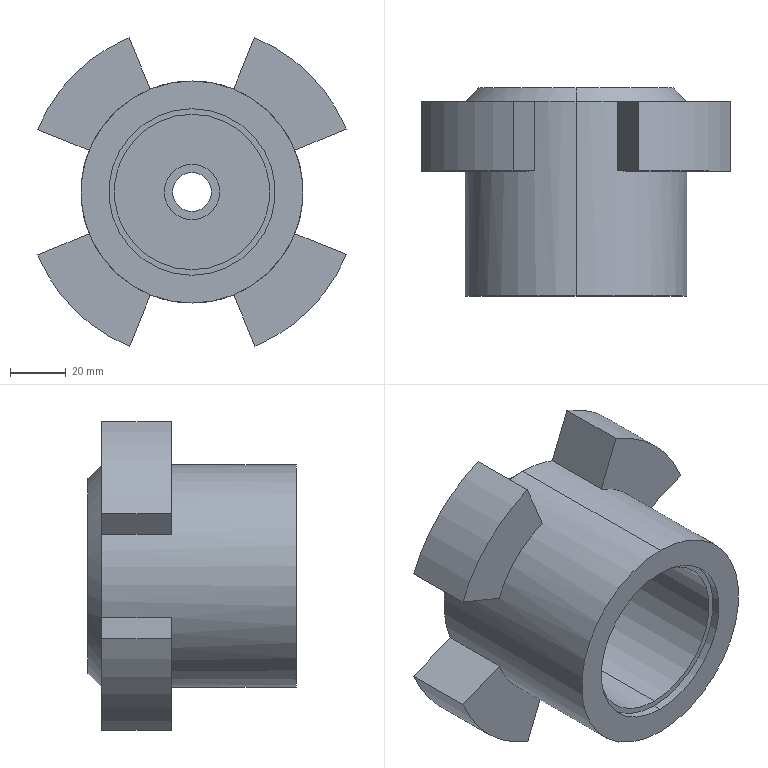Part | SolidWorks | features BaseBody 1 | 1 solid | 37 faces | box 111.243 x 75 x 111.243 mm | volume 319266 mm3 | plane 21 | cylinder 14 | cone 2 | commonest cylinder face diameters 120 x4 14 x2 20 x2 56 x2 60 x2 80 x2
STEP:
#1=CARTESIAN_POINT('',(0.,0.,40.));
#2=VERTEX_POINT('',#1);
#3=CARTESIAN_POINT('',(0.,0.,-40.));
#4=VERTEX_POINT('',#3);
#5=CARTESIAN_POINT('',(0.,0.,0.));
#6=DIRECTION('',(0.,1.,0.));
#7=DIRECTION('',(0.,0.,1.));
#8=AXIS2_PLACEMENT_3D('',#5,#6,#7);
#9=CIRCLE('',#8,40.);
#10=EDGE_CURVE('',#2,#4,#9,.T.);
#11=ORIENTED_EDGE('',*,*,#10,.T.);
#12=CARTESIAN_POINT('',(0.,70.,-40.));
#13=VERTEX_POINT('',#12);
#14=CARTESIAN_POINT('',(0.,45.,-40.));
#15=DIRECTION('',(0.,1.,0.));
#16=VECTOR('',#15,1000.);
#17=LINE('',#14,#16);
#18=EDGE_CURVE('',#4,#13,#17,.T.);
#19=ORIENTED_EDGE('',*,*,#18,.T.);
#20=CARTESIAN_POINT('',(15.,70.,-37.081));
#21=VERTEX_POINT('',#20);
#22=CARTESIAN_POINT('',(0.,70.,0.));
#23=DIRECTION('',(0.,-1.,0.));
#24=DIRECTION('',(0.,0.,1.));
#25=AXIS2_PLACEMENT_3D('',#22,#23,#24);
#26=CIRCLE('',#25,40.);
#27=EDGE_CURVE('',#13,#21,#26,.T.);
#28=ORIENTED_EDGE('',*,*,#27,.T.);
#29=CARTESIAN_POINT('',(15.,45.,-37.081));
#30=VERTEX_POINT('',#29);
#31=CARTESIAN_POINT('',(15.,45.,-37.081));
#32=DIRECTION('',(0.,-1.,0.));
#33=VECTOR('',#32,1000.);
#34=LINE('',#31,#33);
#35=EDGE_CURVE('',#21,#30,#34,.T.);
#36=ORIENTED_EDGE('',*,*,#35,.T.);
#37=CARTESIAN_POINT('',(37.081,45.,-15.));
#38=VERTEX_POINT('',#37);
#39=CARTESIAN_POINT('',(0.,45.,0.));
#40=DIRECTION('',(0.,-1.,0.));
#41=DIRECTION('',(0.,0.,1.));
#42=AXIS2_PLACEMENT_3D('',#39,#40,#41);
#43=CIRCLE('',#42,40.);
#44=EDGE_CURVE('',#30,#38,#43,.T.);
#45=ORIENTED_EDGE('',*,*,#44,.T.);
#46=CARTESIAN_POINT('',(37.081,70.,-15.));
#47=VERTEX_POINT('',#46);
#48=CARTESIAN_POINT('',(37.081,45.,-15.));
#49=DIRECTION('',(0.,1.,0.));
#50=VECTOR('',#49,1000.);
#51=LINE('',#48,#50);
#52=EDGE_CURVE('',#38,#47,#51,.T.);
#53=ORIENTED_EDGE('',*,*,#52,.T.);
#54=CARTESIAN_POINT('',(37.081,70.,15.));
#55=VERTEX_POINT('',#54);
#56=CARTESIAN_POINT('',(0.,70.,0.));
#57=DIRECTION('',(0.,-1.,0.));
#58=DIRECTION('',(0.,0.,1.));
#59=AXIS2_PLACEMENT_3D('',#56,#57,#58);
#60=CIRCLE('',#59,40.);
#61=EDGE_CURVE('',#47,#55,#60,.T.);
#62=ORIENTED_EDGE('',*,*,#61,.T.);
#63=CARTESIAN_POINT('',(37.081,45.,15.));
#64=VERTEX_POINT('',#63);
#65=CARTESIAN_POINT('',(37.081,45.,15.));
#66=DIRECTION('',(0.,-1.,0.));
#67=VECTOR('',#66,1000.);
#68=LINE('',#65,#67);
#69=EDGE_CURVE('',#55,#64,#68,.T.);
#70=ORIENTED_EDGE('',*,*,#69,.T.);
#71=CARTESIAN_POINT('',(15.,45.,37.081));
#72=VERTEX_POINT('',#71);
#73=CARTESIAN_POINT('',(0.,45.,0.));
#74=DIRECTION('',(0.,-1.,0.));
#75=DIRECTION('',(0.,0.,1.));
#76=AXIS2_PLACEMENT_3D('',#73,#74,#75);
#77=CIRCLE('',#76,40.);
#78=EDGE_CURVE('',#64,#72,#77,.T.);
#79=ORIENTED_EDGE('',*,*,#78,.T.);
#80=CARTESIAN_POINT('',(15.,70.,37.081));
#81=VERTEX_POINT('',#80);
#82=CARTESIAN_POINT('',(15.,45.,37.081));
#83=DIRECTION('',(0.,1.,0.));
#84=VECTOR('',#83,1000.);
#85=LINE('',#82,#84);
#86=EDGE_CURVE('',#72,#81,#85,.T.);
#87=ORIENTED_EDGE('',*,*,#86,.T.);
#88=CARTESIAN_POINT('',(0.,70.,40.));
#89=VERTEX_POINT('',#88);
#90=CARTESIAN_POINT('',(0.,70.,0.));
#91=DIRECTION('',(0.,-1.,0.));
#92=DIRECTION('',(0.,0.,1.));
#93=AXIS2_PLACEMENT_3D('',#90,#91,#92);
#94=CIRCLE('',#93,40.);
#95=EDGE_CURVE('',#81,#89,#94,.T.);
#96=ORIENTED_EDGE('',*,*,#95,.T.);
#97=CARTESIAN_POINT('',(0.,45.,40.));
#98=DIRECTION('',(0.,1.,0.));
#99=VECTOR('',#98,1000.);
#100=LINE('',#97,#99);
#101=EDGE_CURVE('',#2,#89,#100,.T.);
#102=ORIENTED_EDGE('',*,*,#101,.F.);
#103=EDGE_LOOP('',(#11,#19,#28,#36,#45,#53,#62,#70,#79,#87,#96,#102));
#104=FACE_OUTER_BOUND('',#103,.T.);
#105=CARTESIAN_POINT('',(0.,45.,0.));
#106=DIRECTION('',(0.,1.,0.));
#107=DIRECTION('',(0.,0.,1.));
#108=AXIS2_PLACEMENT_3D('',#105,#106,#107);
#109=CYLINDRICAL_SURFACE('',#108,40.);
#110=ADVANCED_FACE('',(#104),#109,.T.);
#111=CARTESIAN_POINT('',(0.,75.,-35.));
#112=VERTEX_POINT('',#111);
#113=CARTESIAN_POINT('',(0.,75.,35.));
#114=VERTEX_POINT('',#113);
#115=CARTESIAN_POINT('',(0.,75.,0.));
#116=DIRECTION('',(0.,-1.,0.));
#117=DIRECTION('',(0.,0.,-1.));
#118=AXIS2_PLACEMENT_3D('',#115,#116,#117);
#119=CIRCLE('',#118,35.);
#120=EDGE_CURVE('',#112,#114,#119,.T.);
#121=ORIENTED_EDGE('',*,*,#120,.T.);
#122=CARTESIAN_POINT('',(0.,70.,40.));
#123=DIRECTION('',(0.,-0.7071,0.7071));
#124=VECTOR('',#123,1000.);
#125=LINE('',#122,#124);
#126=EDGE_CURVE('',#114,#89,#125,.T.);
#127=ORIENTED_EDGE('',*,*,#126,.T.);
#128=ORIENTED_EDGE('',*,*,#95,.F.);
#129=CARTESIAN_POINT('',(0.,70.,0.));
#130=DIRECTION('',(0.,1.,0.));
#131=DIRECTION('',(0.,0.,-1.));
#132=AXIS2_PLACEMENT_3D('',#129,#130,#131);
#133=CIRCLE('',#132,40.);
#134=EDGE_CURVE('',#81,#55,#133,.T.);
#135=ORIENTED_EDGE('',*,*,#134,.T.);
#136=ORIENTED_EDGE('',*,*,#61,.F.);
#137=CARTESIAN_POINT('',(0.,70.,0.));
#138=DIRECTION('',(0.,1.,0.));
#139=DIRECTION('',(0.,0.,-1.));
#140=AXIS2_PLACEMENT_3D('',#137,#138,#139);
#141=CIRCLE('',#140,40.);
#142=EDGE_CURVE('',#47,#21,#141,.T.);
#143=ORIENTED_EDGE('',*,*,#142,.T.);
#144=ORIENTED_EDGE('',*,*,#27,.F.);
#145=CARTESIAN_POINT('',(0.,70.,-40.));
#146=DIRECTION('',(0.,-0.7071,-0.7071));
#147=VECTOR('',#146,1000.);
#148=LINE('',#145,#147);
#149=EDGE_CURVE('',#112,#13,#148,.T.);
#150=ORIENTED_EDGE('',*,*,#149,.F.);
#151=EDGE_LOOP('',(#121,#127,#128,#135,#136,#143,#144,#150));
#152=FACE_OUTER_BOUND('',#151,.T.);
#153=CARTESIAN_POINT('',(0.,70.,0.));
#154=DIRECTION('',(0.,-1.,0.));
#155=DIRECTION('',(0.,0.,-1.));
#156=AXIS2_PLACEMENT_3D('',#153,#154,#155);
#157=CONICAL_SURFACE('',#156,40.,0.7854);
#158=ADVANCED_FACE('',(#152),#157,.T.);
#159=CARTESIAN_POINT('',(0.,3.,30.));
#160=VERTEX_POINT('',#159);
#161=CARTESIAN_POINT('',(0.,3.,-30.));
#162=VERTEX_POINT('',#161);
#163=CARTESIAN_POINT('',(0.,3.,0.));
#164=DIRECTION('',(0.,-1.,0.));
#165=DIRECTION('',(0.,0.,-1.));
#166=AXIS2_PLACEMENT_3D('',#163,#164,#165);
#167=CIRCLE('',#166,30.);
#168=EDGE_CURVE('',#160,#162,#167,.T.);
#169=ORIENTED_EDGE('',*,*,#168,.F.);
#170=CARTESIAN_POINT('',(0.,0.,30.));
#171=VERTEX_POINT('',#170);
#172=CARTESIAN_POINT('',(0.,3.,30.));
#173=DIRECTION('',(0.,-1.,0.));
#174=VECTOR('',#173,1000.);
#175=LINE('',#172,#174);
#176=EDGE_CURVE('',#160,#171,#175,.T.);
#177=ORIENTED_EDGE('',*,*,#176,.T.);
#178=CARTESIAN_POINT('',(0.,0.,-30.));
#179=VERTEX_POINT('',#178);
#180=CARTESIAN_POINT('',(0.,0.,0.));
#181=DIRECTION('',(0.,-1.,0.));
#182=DIRECTION('',(0.,0.,-1.));
#183=AXIS2_PLACEMENT_3D('',#180,#181,#182);
#184=CIRCLE('',#183,30.);
#185=EDGE_CURVE('',#171,#179,#184,.T.);
#186=ORIENTED_EDGE('',*,*,#185,.T.);
#187=CARTESIAN_POINT('',(0.,3.,-30.));
#188=DIRECTION('',(0.,-1.,0.));
#189=VECTOR('',#188,1000.);
#190=LINE('',#187,#189);
#191=EDGE_CURVE('',#162,#179,#190,.T.);
#192=ORIENTED_EDGE('',*,*,#191,.F.);
#193=EDGE_LOOP('',(#169,#177,#186,#192));
#194=FACE_OUTER_BOUND('',#193,.T.);
#195=CARTESIAN_POINT('',(0.,3.,0.));
#196=DIRECTION('',(0.,-1.,0.));
#197=DIRECTION('',(0.,0.,-1.));
#198=AXIS2_PLACEMENT_3D('',#195,#196,#197);
#199=CYLINDRICAL_SURFACE('',#198,30.);
#200=ADVANCED_FACE('',(#194),#199,.F.);
#201=CARTESIAN_POINT('',(0.,51.,-7.));
#202=VERTEX_POINT('',#201);
#203=CARTESIAN_POINT('',(0.,51.,7.));
#204=VERTEX_POINT('',#203);
#205=CARTESIAN_POINT('',(0.,51.,0.));
#206=DIRECTION('',(0.,1.,0.));
#207=DIRECTION('',(0.,0.,1.));
#208=AXIS2_PLACEMENT_3D('',#205,#206,#207);
#209=CIRCLE('',#208,7.);
#210=EDGE_CURVE('',#202,#204,#209,.T.);
#211=ORIENTED_EDGE('',*,*,#210,.F.);
#212=CARTESIAN_POINT('',(0.,75.,-7.));
#213=VERTEX_POINT('',#212);
#214=CARTESIAN_POINT('',(0.,75.,-7.));
#215=DIRECTION('',(0.,1.,0.));
#216=VECTOR('',#215,1000.);
#217=LINE('',#214,#216);
#218=EDGE_CURVE('',#202,#213,#217,.T.);
#219=ORIENTED_EDGE('',*,*,#218,.T.);
#220=CARTESIAN_POINT('',(0.,75.,7.));
#221=VERTEX_POINT('',#220);
#222=CARTESIAN_POINT('',(0.,75.,0.));
#223=DIRECTION('',(0.,-1.,0.));
#224=DIRECTION('',(0.,0.,1.));
#225=AXIS2_PLACEMENT_3D('',#222,#223,#224);
#226=CIRCLE('',#225,7.);
#227=EDGE_CURVE('',#221,#213,#226,.T.);
#228=ORIENTED_EDGE('',*,*,#227,.F.);
#229=CARTESIAN_POINT('',(0.,75.,7.));
#230=DIRECTION('',(0.,1.,0.));
#231=VECTOR('',#230,1000.);
#232=LINE('',#229,#231);
#233=EDGE_CURVE('',#204,#221,#232,.T.);
#234=ORIENTED_EDGE('',*,*,#233,.F.);
#235=EDGE_LOOP('',(#211,#219,#228,#234));
#236=FACE_OUTER_BOUND('',#235,.T.);
#237=CARTESIAN_POINT('',(0.,75.,0.));
#238=DIRECTION('',(0.,1.,0.));
#239=DIRECTION('',(0.,0.,1.));
#240=AXIS2_PLACEMENT_3D('',#237,#238,#239);
#241=CYLINDRICAL_SURFACE('',#240,7.);
#242=ADVANCED_FACE('',(#236),#241,.F.);
#243=CARTESIAN_POINT('',(0.,53.,28.));
#244=VERTEX_POINT('',#243);
#245=CARTESIAN_POINT('',(0.,53.,-28.));
#246=VERTEX_POINT('',#245);
#247=CARTESIAN_POINT('',(0.,53.,0.));
#248=DIRECTION('',(0.,-1.,0.));
#249=DIRECTION('',(0.,0.,-1.));
#250=AXIS2_PLACEMENT_3D('',#247,#248,#249);
#251=CIRCLE('',#250,28.);
#252=EDGE_CURVE('',#244,#246,#251,.T.);
#253=ORIENTED_EDGE('',*,*,#252,.F.);
#254=CARTESIAN_POINT('',(0.,3.,28.));
#255=VERTEX_POINT('',#254);
#256=CARTESIAN_POINT('',(0.,51.,28.));
#257=DIRECTION('',(0.,-1.,0.));
#258=VECTOR('',#257,1000.);
#259=LINE('',#256,#258);
#260=EDGE_CURVE('',#244,#255,#259,.T.);
#261=ORIENTED_EDGE('',*,*,#260,.T.);
#262=CARTESIAN_POINT('',(0.,3.,-28.));
#263=VERTEX_POINT('',#262);
#264=CARTESIAN_POINT('',(0.,3.,0.));
#265=DIRECTION('',(0.,1.,0.));
#266=DIRECTION('',(0.,0.,-1.));
#267=AXIS2_PLACEMENT_3D('',#264,#265,#266);
#268=CIRCLE('',#267,28.);
#269=EDGE_CURVE('',#263,#255,#268,.T.);
#270=ORIENTED_EDGE('',*,*,#269,.F.);
#271=CARTESIAN_POINT('',(0.,51.,-28.));
#272=DIRECTION('',(0.,-1.,0.));
#273=VECTOR('',#272,1000.);
#274=LINE('',#271,#273);
#275=EDGE_CURVE('',#246,#263,#274,.T.);
#276=ORIENTED_EDGE('',*,*,#275,.F.);
#277=EDGE_LOOP('',(#253,#261,#270,#276));
#278=FACE_OUTER_BOUND('',#277,.T.);
#279=CARTESIAN_POINT('',(0.,51.,0.));
#280=DIRECTION('',(0.,-1.,0.));
#281=DIRECTION('',(0.,0.,-1.));
#282=AXIS2_PLACEMENT_3D('',#279,#280,#281);
#283=CYLINDRICAL_SURFACE('',#282,28.);
#284=ADVANCED_FACE('',(#278),#283,.F.);
#285=CARTESIAN_POINT('',(0.,53.,-10.));
#286=VERTEX_POINT('',#285);
#287=CARTESIAN_POINT('',(0.,53.,10.));
#288=VERTEX_POINT('',#287);
#289=CARTESIAN_POINT('',(0.,53.,0.));
#290=DIRECTION('',(0.,-1.,0.));
#291=DIRECTION('',(0.,0.,-1.));
#292=AXIS2_PLACEMENT_3D('',#289,#290,#291);
#293=CIRCLE('',#292,10.);
#294=EDGE_CURVE('',#286,#288,#293,.T.);
#295=ORIENTED_EDGE('',*,*,#294,.T.);
#296=CARTESIAN_POINT('',(0.,51.,10.));
#297=VERTEX_POINT('',#296);
#298=CARTESIAN_POINT('',(0.,53.,10.));
#299=DIRECTION('',(0.,-1.,0.));
#300=VECTOR('',#299,1000.);
#301=LINE('',#298,#300);
#302=EDGE_CURVE('',#288,#297,#301,.T.);
#303=ORIENTED_EDGE('',*,*,#302,.T.);
#304=CARTESIAN_POINT('',(0.,51.,-10.));
#305=VERTEX_POINT('',#304);
#306=CARTESIAN_POINT('',(0.,51.,0.));
#307=DIRECTION('',(0.,-1.,0.));
#308=DIRECTION('',(0.,0.,-1.));
#309=AXIS2_PLACEMENT_3D('',#306,#307,#308);
#310=CIRCLE('',#309,10.);
#311=EDGE_CURVE('',#305,#297,#310,.T.);
#312=ORIENTED_EDGE('',*,*,#311,.F.);
#313=CARTESIAN_POINT('',(0.,53.,-10.));
#314=DIRECTION('',(0.,-1.,0.));
#315=VECTOR('',#314,1000.);
#316=LINE('',#313,#315);
#317=EDGE_CURVE('',#286,#305,#316,.T.);
#318=ORIENTED_EDGE('',*,*,#317,.F.);
#319=EDGE_LOOP('',(#295,#303,#312,#318));
#320=FACE_OUTER_BOUND('',#319,.T.);
#321=CARTESIAN_POINT('',(0.,53.,0.));
#322=DIRECTION('',(0.,-1.,0.));
#323=DIRECTION('',(0.,0.,-1.));
#324=AXIS2_PLACEMENT_3D('',#321,#322,#323);
#325=CYLINDRICAL_SURFACE('',#324,10.);
#326=ADVANCED_FACE('',(#320),#325,.T.);
#327=ORIENTED_EDGE('',*,*,#18,.F.);
#328=CARTESIAN_POINT('',(0.,0.,0.));
#329=DIRECTION('',(0.,1.,0.));
#330=DIRECTION('',(0.,0.,1.));
#331=AXIS2_PLACEMENT_3D('',#328,#329,#330);
#332=CIRCLE('',#331,40.);
#333=EDGE_CURVE('',#4,#2,#332,.T.);
#334=ORIENTED_EDGE('',*,*,#333,.T.);
#335=ORIENTED_EDGE('',*,*,#101,.T.);
#336=CARTESIAN_POINT('',(-15.,70.,37.081));
#337=VERTEX_POINT('',#336);
#338=CARTESIAN_POINT('',(0.,70.,0.));
#339=DIRECTION('',(0.,-1.,0.));
#340=DIRECTION('',(0.,0.,1.));
#341=AXIS2_PLACEMENT_3D('',#338,#339,#340);
#342=CIRCLE('',#341,40.);
#343=EDGE_CURVE('',#89,#337,#342,.T.);
#344=ORIENTED_EDGE('',*,*,#343,.T.);
#345=CARTESIAN_POINT('',(-15.,45.,37.081));
#346=VERTEX_POINT('',#345);
#347=CARTESIAN_POINT('',(-15.,45.,37.081));
#348=DIRECTION('',(0.,-1.,0.));
#349=VECTOR('',#348,1000.);
#350=LINE('',#347,#349);
#351=EDGE_CURVE('',#337,#346,#350,.T.);
#352=ORIENTED_EDGE('',*,*,#351,.T.);
#353=CARTESIAN_POINT('',(-37.081,45.,15.));
#354=VERTEX_POINT('',#353);
#355=CARTESIAN_POINT('',(0.,45.,0.));
#356=DIRECTION('',(0.,-1.,0.));
#357=DIRECTION('',(0.,0.,1.));
#358=AXIS2_PLACEMENT_3D('',#355,#356,#357);
#359=CIRCLE('',#358,40.);
#360=EDGE_CURVE('',#346,#354,#359,.T.);
#361=ORIENTED_EDGE('',*,*,#360,.T.);
#362=CARTESIAN_POINT('',(-37.081,70.,15.));
#363=VERTEX_POINT('',#362);
#364=CARTESIAN_POINT('',(-37.081,45.,15.));
#365=DIRECTION('',(0.,1.,0.));
#366=VECTOR('',#365,1000.);
#367=LINE('',#364,#366);
#368=EDGE_CURVE('',#354,#363,#367,.T.);
#369=ORIENTED_EDGE('',*,*,#368,.T.);
#370=CARTESIAN_POINT('',(-37.081,70.,-15.));
#371=VERTEX_POINT('',#370);
#372=CARTESIAN_POINT('',(0.,70.,0.));
#373=DIRECTION('',(0.,-1.,0.));
#374=DIRECTION('',(0.,0.,1.));
#375=AXIS2_PLACEMENT_3D('',#372,#373,#374);
#376=CIRCLE('',#375,40.);
#377=EDGE_CURVE('',#363,#371,#376,.T.);
#378=ORIENTED_EDGE('',*,*,#377,.T.);
#379=CARTESIAN_POINT('',(-37.081,45.,-15.));
#380=VERTEX_POINT('',#379);
#381=CARTESIAN_POINT('',(-37.081,45.,-15.));
#382=DIRECTION('',(0.,-1.,0.));
#383=VECTOR('',#382,1000.);
#384=LINE('',#381,#383);
#385=EDGE_CURVE('',#371,#380,#384,.T.);
#386=ORIENTED_EDGE('',*,*,#385,.T.);
#387=CARTESIAN_POINT('',(-15.,45.,-37.081));
#388=VERTEX_POINT('',#387);
#389=CARTESIAN_POINT('',(0.,45.,0.));
#390=DIRECTION('',(0.,-1.,0.));
#391=DIRECTION('',(0.,0.,1.));
#392=AXIS2_PLACEMENT_3D('',#389,#390,#391);
#393=CIRCLE('',#392,40.);
#394=EDGE_CURVE('',#380,#388,#393,.T.);
#395=ORIENTED_EDGE('',*,*,#394,.T.);
#396=CARTESIAN_POINT('',(-15.,70.,-37.081));
#397=VERTEX_POINT('',#396);
#398=CARTESIAN_POINT('',(-15.,45.,-37.081));
#399=DIRECTION('',(0.,1.,0.));
#400=VECTOR('',#399,1000.);
#401=LINE('',#398,#400);
#402=EDGE_CURVE('',#388,#397,#401,.T.);
#403=ORIENTED_EDGE('',*,*,#402,.T.);
#404=CARTESIAN_POINT('',(0.,70.,0.));
#405=DIRECTION('',(0.,-1.,0.));
#406=DIRECTION('',(0.,0.,1.));
#407=AXIS2_PLACEMENT_3D('',#404,#405,#406);
#408=CIRCLE('',#407,40.);
#409=EDGE_CURVE('',#397,#13,#408,.T.);
#410=ORIENTED_EDGE('',*,*,#409,.T.);
#411=EDGE_LOOP('',(#327,#334,#335,#344,#352,#361,#369,#378,#386,#395,#403,#410));
#412=FACE_OUTER_BOUND('',#411,.T.);
#413=CARTESIAN_POINT('',(0.,45.,0.));
#414=DIRECTION('',(0.,1.,0.));
#415=DIRECTION('',(0.,0.,1.));
#416=AXIS2_PLACEMENT_3D('',#413,#414,#415);
#417=CYLINDRICAL_SURFACE('',#416,40.);
#418=ADVANCED_FACE('',(#412),#417,.T.);
#419=ORIENTED_EDGE('',*,*,#126,.F.);
#420=CARTESIAN_POINT('',(0.,75.,0.));
#421=DIRECTION('',(0.,-1.,0.));
#422=DIRECTION('',(0.,0.,-1.));
#423=AXIS2_PLACEMENT_3D('',#420,#421,#422);
#424=CIRCLE('',#423,35.);
#425=EDGE_CURVE('',#114,#112,#424,.T.);
#426=ORIENTED_EDGE('',*,*,#425,.T.);
#427=ORIENTED_EDGE('',*,*,#149,.T.);
#428=ORIENTED_EDGE('',*,*,#409,.F.);
#429=CARTESIAN_POINT('',(0.,70.,0.));
#430=DIRECTION('',(0.,1.,0.));
#431=DIRECTION('',(0.,0.,-1.));
#432=AXIS2_PLACEMENT_3D('',#429,#430,#431);
#433=CIRCLE('',#432,40.);
#434=EDGE_CURVE('',#397,#371,#433,.T.);
#435=ORIENTED_EDGE('',*,*,#434,.T.);
#436=ORIENTED_EDGE('',*,*,#377,.F.);
#437=CARTESIAN_POINT('',(0.,70.,0.));
#438=DIRECTION('',(0.,1.,0.));
#439=DIRECTION('',(0.,0.,-1.));
#440=AXIS2_PLACEMENT_3D('',#437,#438,#439);
#441=CIRCLE('',#440,40.);
#442=EDGE_CURVE('',#363,#337,#441,.T.);
#443=ORIENTED_EDGE('',*,*,#442,.T.);
#444=ORIENTED_EDGE('',*,*,#343,.F.);
#445=EDGE_LOOP('',(#419,#426,#427,#428,#435,#436,#443,#444));
#446=FACE_OUTER_BOUND('',#445,.T.);
#447=CARTESIAN_POINT('',(0.,70.,0.));
#448=DIRECTION('',(0.,-1.,0.));
#449=DIRECTION('',(0.,0.,-1.));
#450=AXIS2_PLACEMENT_3D('',#447,#448,#449);
#451=CONICAL_SURFACE('',#450,40.,0.7854);
#452=ADVANCED_FACE('',(#446),#451,.T.);
#453=ORIENTED_EDGE('',*,*,#402,.F.);
#454=CARTESIAN_POINT('',(-22.5,45.,-55.621));
#455=VERTEX_POINT('',#454);
#456=CARTESIAN_POINT('',(-22.5,45.,-55.621));
#457=DIRECTION('',(0.375,0.,0.927));
#458=VECTOR('',#457,1000.);
#459=LINE('',#456,#458);
#460=EDGE_CURVE('',#455,#388,#459,.T.);
#461=ORIENTED_EDGE('',*,*,#460,.F.);
#462=CARTESIAN_POINT('',(-22.5,70.,-55.621));
#463=VERTEX_POINT('',#462);
#464=CARTESIAN_POINT('',(-22.5,45.,-55.621));
#465=DIRECTION('',(0.,-1.,0.));
#466=VECTOR('',#465,1000.);
#467=LINE('',#464,#466);
#468=EDGE_CURVE('',#463,#455,#467,.T.);
#469=ORIENTED_EDGE('',*,*,#468,.F.);
#470=CARTESIAN_POINT('',(-22.5,70.,-55.621));
#471=DIRECTION('',(-0.375,0.,-0.927));
#472=VECTOR('',#471,1000.);
#473=LINE('',#470,#472);
#474=EDGE_CURVE('',#397,#463,#473,.T.);
#475=ORIENTED_EDGE('',*,*,#474,.F.);
#476=EDGE_LOOP('',(#453,#461,#469,#475));
#477=FACE_OUTER_BOUND('',#476,.T.);
#478=CARTESIAN_POINT('',(-22.5,45.,-55.621));
#479=DIRECTION('',(-0.927,0.,0.375));
#480=DIRECTION('',(0.375,0.,0.927));
#481=AXIS2_PLACEMENT_3D('',#478,#479,#480);
#482=PLANE('',#481);
#483=ADVANCED_FACE('',(#477),#482,.F.);
#484=ORIENTED_EDGE('',*,*,#394,.F.);
#485=CARTESIAN_POINT('',(-55.54,45.,-22.7));
#486=VERTEX_POINT('',#485);
#487=CARTESIAN_POINT('',(-37.081,45.,-15.));
#488=DIRECTION('',(-0.9229,0.,-0.385));
#489=VECTOR('',#488,1000.);
#490=LINE('',#487,#489);
#491=EDGE_CURVE('',#380,#486,#490,.T.);
#492=ORIENTED_EDGE('',*,*,#491,.T.);
#493=CARTESIAN_POINT('',(0.,45.,0.));
#494=DIRECTION('',(0.,-1.,0.));
#495=DIRECTION('',(0.,0.,-1.));
#496=AXIS2_PLACEMENT_3D('',#493,#494,#495);
#497=CIRCLE('',#496,60.);
#498=EDGE_CURVE('',#486,#455,#497,.T.);
#499=ORIENTED_EDGE('',*,*,#498,.T.);
#500=ORIENTED_EDGE('',*,*,#460,.T.);
#501=EDGE_LOOP('',(#484,#492,#499,#500));
#502=FACE_OUTER_BOUND('',#501,.T.);
#503=CARTESIAN_POINT('',(0.,45.,0.));
#504=DIRECTION('',(0.,-1.,0.));
#505=DIRECTION('',(0.,0.,-1.));
#506=AXIS2_PLACEMENT_3D('',#503,#504,#505);
#507=PLANE('',#506);
#508=ADVANCED_FACE('',(#502),#507,.T.);
#509=CARTESIAN_POINT('',(-55.54,70.,-22.7));
#510=VERTEX_POINT('',#509);
#511=CARTESIAN_POINT('',(-55.54,45.,-22.7));
#512=DIRECTION('',(0.,1.,0.));
#513=VECTOR('',#512,1000.);
#514=LINE('',#511,#513);
#515=EDGE_CURVE('',#486,#510,#514,.T.);
#516=ORIENTED_EDGE('',*,*,#515,.F.);
#517=ORIENTED_EDGE('',*,*,#491,.F.);
#518=ORIENTED_EDGE('',*,*,#385,.F.);
#519=CARTESIAN_POINT('',(-55.54,70.,-22.7));
#520=DIRECTION('',(0.9229,0.,0.385));
#521=VECTOR('',#520,1000.);
#522=LINE('',#519,#521);
#523=EDGE_CURVE('',#510,#371,#522,.T.);
#524=ORIENTED_EDGE('',*,*,#523,.F.);
#525=EDGE_LOOP('',(#516,#517,#518,#524));
#526=FACE_OUTER_BOUND('',#525,.T.);
#527=CARTESIAN_POINT('',(-55.54,45.,-22.7));
#528=DIRECTION('',(0.385,0.,-0.9229));
#529=DIRECTION('',(-0.9229,0.,-0.385));
#530=AXIS2_PLACEMENT_3D('',#527,#528,#529);
#531=PLANE('',#530);
#532=ADVANCED_FACE('',(#526),#531,.F.);
#533=ORIENTED_EDGE('',*,*,#368,.F.);
#534=CARTESIAN_POINT('',(-55.621,45.,22.5));
#535=VERTEX_POINT('',#534);
#536=CARTESIAN_POINT('',(-55.621,45.,22.5));
#537=DIRECTION('',(0.927,0.,-0.375));
#538=VECTOR('',#537,1000.);
#539=LINE('',#536,#538);
#540=EDGE_CURVE('',#535,#354,#539,.T.);
#541=ORIENTED_EDGE('',*,*,#540,.F.);
#542=CARTESIAN_POINT('',(-55.621,70.,22.5));
#543=VERTEX_POINT('',#542);
#544=CARTESIAN_POINT('',(-55.621,45.,22.5));
#545=DIRECTION('',(0.,-1.,0.));
#546=VECTOR('',#545,1000.);
#547=LINE('',#544,#546);
#548=EDGE_CURVE('',#543,#535,#547,.T.);
#549=ORIENTED_EDGE('',*,*,#548,.F.);
#550=CARTESIAN_POINT('',(-55.621,70.,22.5));
#551=DIRECTION('',(-0.927,0.,0.375));
#552=VECTOR('',#551,1000.);
#553=LINE('',#550,#552);
#554=EDGE_CURVE('',#363,#543,#553,.T.);
#555=ORIENTED_EDGE('',*,*,#554,.F.);
#556=EDGE_LOOP('',(#533,#541,#549,#555));
#557=FACE_OUTER_BOUND('',#556,.T.);
#558=CARTESIAN_POINT('',(-55.621,45.,22.5));
#559=DIRECTION('',(0.375,0.,0.927));
#560=DIRECTION('',(0.927,0.,-0.375));
#561=AXIS2_PLACEMENT_3D('',#558,#559,#560);
#562=PLANE('',#561);
#563=ADVANCED_FACE('',(#557),#562,.F.);
#564=ORIENTED_EDGE('',*,*,#360,.F.);
#565=CARTESIAN_POINT('',(-22.7,45.,55.54));
#566=VERTEX_POINT('',#565);
#567=CARTESIAN_POINT('',(-15.,45.,37.081));
#568=DIRECTION('',(-0.385,0.,0.9229));
#569=VECTOR('',#568,1000.);
#570=LINE('',#567,#569);
#571=EDGE_CURVE('',#346,#566,#570,.T.);
#572=ORIENTED_EDGE('',*,*,#571,.T.);
#573=CARTESIAN_POINT('',(0.,45.,0.));
#574=DIRECTION('',(0.,-1.,0.));
#575=DIRECTION('',(0.,0.,-1.));
#576=AXIS2_PLACEMENT_3D('',#573,#574,#575);
#577=CIRCLE('',#576,60.);
#578=EDGE_CURVE('',#566,#535,#577,.T.);
#579=ORIENTED_EDGE('',*,*,#578,.T.);
#580=ORIENTED_EDGE('',*,*,#540,.T.);
#581=EDGE_LOOP('',(#564,#572,#579,#580));
#582=FACE_OUTER_BOUND('',#581,.T.);
#583=CARTESIAN_POINT('',(0.,45.,0.));
#584=DIRECTION('',(0.,-1.,0.));
#585=DIRECTION('',(0.,0.,-1.));
#586=AXIS2_PLACEMENT_3D('',#583,#584,#585);
#587=PLANE('',#586);
#588=ADVANCED_FACE('',(#582),#587,.T.);
#589=CARTESIAN_POINT('',(-22.7,70.,55.54));
#590=VERTEX_POINT('',#589);
#591=CARTESIAN_POINT('',(-22.7,45.,55.54));
#592=DIRECTION('',(0.,1.,0.));
#593=VECTOR('',#592,1000.);
#594=LINE('',#591,#593);
#595=EDGE_CURVE('',#566,#590,#594,.T.);
#596=ORIENTED_EDGE('',*,*,#595,.F.);
#597=ORIENTED_EDGE('',*,*,#571,.F.);
#598=ORIENTED_EDGE('',*,*,#351,.F.);
#599=CARTESIAN_POINT('',(-22.7,70.,55.54));
#600=DIRECTION('',(0.385,0.,-0.9229));
#601=VECTOR('',#600,1000.);
#602=LINE('',#599,#601);
#603=EDGE_CURVE('',#590,#337,#602,.T.);
#604=ORIENTED_EDGE('',*,*,#603,.F.);
#605=EDGE_LOOP('',(#596,#597,#598,#604));
#606=FACE_OUTER_BOUND('',#605,.T.);
#607=CARTESIAN_POINT('',(-22.7,45.,55.54));
#608=DIRECTION('',(-0.9229,0.,-0.385));
#609=DIRECTION('',(-0.385,0.,0.9229));
#610=AXIS2_PLACEMENT_3D('',#607,#608,#609);
#611=PLANE('',#610);
#612=ADVANCED_FACE('',(#606),#611,.F.);
#613=CARTESIAN_POINT('',(0.,0.,0.));
#614=DIRECTION('',(0.,-1.,0.));
#615=DIRECTION('',(0.,0.,-1.));
#616=AXIS2_PLACEMENT_3D('',#613,#614,#615);
#617=CIRCLE('',#616,30.);
#618=EDGE_CURVE('',#179,#171,#617,.T.);
#619=ORIENTED_EDGE('',*,*,#618,.F.);
#620=ORIENTED_EDGE('',*,*,#185,.F.);
#621=EDGE_LOOP('',(#619,#620));
#622=FACE_BOUND('',#621,.T.);
#623=ORIENTED_EDGE('',*,*,#10,.F.);
#624=ORIENTED_EDGE('',*,*,#333,.F.);
#625=EDGE_LOOP('',(#623,#624));
#626=FACE_OUTER_BOUND('',#625,.T.);
#627=CARTESIAN_POINT('',(0.,0.,0.));
#628=DIRECTION('',(0.,1.,0.));
#629=DIRECTION('',(0.,0.,1.));
#630=AXIS2_PLACEMENT_3D('',#627,#628,#629);
#631=PLANE('',#630);
#632=ADVANCED_FACE('',(#622,#626),#631,.F.);
#633=ORIENTED_EDGE('',*,*,#603,.T.);
#634=ORIENTED_EDGE('',*,*,#442,.F.);
#635=ORIENTED_EDGE('',*,*,#554,.T.);
#636=CARTESIAN_POINT('',(0.,70.,0.));
#637=DIRECTION('',(0.,1.,0.));
#638=DIRECTION('',(0.,0.,-1.));
#639=AXIS2_PLACEMENT_3D('',#636,#637,#638);
#640=CIRCLE('',#639,60.);
#641=EDGE_CURVE('',#543,#590,#640,.T.);
#642=ORIENTED_EDGE('',*,*,#641,.T.);
#643=EDGE_LOOP('',(#633,#634,#635,#642));
#644=FACE_OUTER_BOUND('',#643,.T.);
#645=CARTESIAN_POINT('',(0.,70.,0.));
#646=DIRECTION('',(0.,1.,0.));
#647=DIRECTION('',(0.,0.,1.));
#648=AXIS2_PLACEMENT_3D('',#645,#646,#647);
#649=PLANE('',#648);
#650=ADVANCED_FACE('',(#644),#649,.T.);
#651=ORIENTED_EDGE('',*,*,#523,.T.);
#652=ORIENTED_EDGE('',*,*,#434,.F.);
#653=ORIENTED_EDGE('',*,*,#474,.T.);
#654=CARTESIAN_POINT('',(0.,70.,0.));
#655=DIRECTION('',(0.,1.,0.));
#656=DIRECTION('',(0.,0.,-1.));
#657=AXIS2_PLACEMENT_3D('',#654,#655,#656);
#658=CIRCLE('',#657,60.);
#659=EDGE_CURVE('',#463,#510,#658,.T.);
#660=ORIENTED_EDGE('',*,*,#659,.T.);
#661=EDGE_LOOP('',(#651,#652,#653,#660));
#662=FACE_OUTER_BOUND('',#661,.T.);
#663=CARTESIAN_POINT('',(0.,70.,0.));
#664=DIRECTION('',(0.,1.,0.));
#665=DIRECTION('',(0.,0.,1.));
#666=AXIS2_PLACEMENT_3D('',#663,#664,#665);
#667=PLANE('',#666);
#668=ADVANCED_FACE('',(#662),#667,.T.);
#669=ORIENTED_EDGE('',*,*,#227,.T.);
#670=CARTESIAN_POINT('',(0.,75.,0.));
#671=DIRECTION('',(0.,-1.,0.));
#672=DIRECTION('',(0.,0.,1.));
#673=AXIS2_PLACEMENT_3D('',#670,#671,#672);
#674=CIRCLE('',#673,7.);
#675=EDGE_CURVE('',#213,#221,#674,.T.);
#676=ORIENTED_EDGE('',*,*,#675,.T.);
#677=EDGE_LOOP('',(#669,#676));
#678=FACE_BOUND('',#677,.T.);
#679=ORIENTED_EDGE('',*,*,#120,.F.);
#680=ORIENTED_EDGE('',*,*,#425,.F.);
#681=EDGE_LOOP('',(#679,#680));
#682=FACE_OUTER_BOUND('',#681,.T.);
#683=CARTESIAN_POINT('',(0.,75.,0.));
#684=DIRECTION('',(0.,1.,0.));
#685=DIRECTION('',(0.,0.,1.));
#686=AXIS2_PLACEMENT_3D('',#683,#684,#685);
#687=PLANE('',#686);
#688=ADVANCED_FACE('',(#678,#682),#687,.T.);
#689=ORIENTED_EDGE('',*,*,#659,.F.);
#690=ORIENTED_EDGE('',*,*,#468,.T.);
#691=ORIENTED_EDGE('',*,*,#498,.F.);
#692=ORIENTED_EDGE('',*,*,#515,.T.);
#693=EDGE_LOOP('',(#689,#690,#691,#692));
#694=FACE_OUTER_BOUND('',#693,.T.);
#695=CARTESIAN_POINT('',(0.,75.,0.));
#696=DIRECTION('',(0.,-1.,0.));
#697=DIRECTION('',(0.,0.,-1.));
#698=AXIS2_PLACEMENT_3D('',#695,#696,#697);
#699=CYLINDRICAL_SURFACE('',#698,60.);
#700=ADVANCED_FACE('',(#694),#699,.T.);
#701=ORIENTED_EDGE('',*,*,#641,.F.);
#702=ORIENTED_EDGE('',*,*,#548,.T.);
#703=ORIENTED_EDGE('',*,*,#578,.F.);
#704=ORIENTED_EDGE('',*,*,#595,.T.);
#705=EDGE_LOOP('',(#701,#702,#703,#704));
#706=FACE_OUTER_BOUND('',#705,.T.);
#707=CARTESIAN_POINT('',(0.,75.,0.));
#708=DIRECTION('',(0.,-1.,0.));
#709=DIRECTION('',(0.,0.,-1.));
#710=AXIS2_PLACEMENT_3D('',#707,#708,#709);
#711=CYLINDRICAL_SURFACE('',#710,60.);
#712=ADVANCED_FACE('',(#706),#711,.T.);
#713=ORIENTED_EDGE('',*,*,#86,.F.);
#714=CARTESIAN_POINT('',(22.5,45.,55.621));
#715=VERTEX_POINT('',#714);
#716=CARTESIAN_POINT('',(22.5,45.,55.621));
#717=DIRECTION('',(-0.375,0.,-0.927));
#718=VECTOR('',#717,1000.);
#719=LINE('',#716,#718);
#720=EDGE_CURVE('',#715,#72,#719,.T.);
#721=ORIENTED_EDGE('',*,*,#720,.F.);
#722=CARTESIAN_POINT('',(22.5,70.,55.621));
#723=VERTEX_POINT('',#722);
#724=CARTESIAN_POINT('',(22.5,45.,55.621));
#725=DIRECTION('',(0.,-1.,0.));
#726=VECTOR('',#725,1000.);
#727=LINE('',#724,#726);
#728=EDGE_CURVE('',#723,#715,#727,.T.);
#729=ORIENTED_EDGE('',*,*,#728,.F.);
#730=CARTESIAN_POINT('',(22.5,70.,55.621));
#731=DIRECTION('',(0.375,0.,0.927));
#732=VECTOR('',#731,1000.);
#733=LINE('',#730,#732);
#734=EDGE_CURVE('',#81,#723,#733,.T.);
#735=ORIENTED_EDGE('',*,*,#734,.F.);
#736=EDGE_LOOP('',(#713,#721,#729,#735));
#737=FACE_OUTER_BOUND('',#736,.T.);
#738=CARTESIAN_POINT('',(22.5,45.,55.621));
#739=DIRECTION('',(0.927,0.,-0.375));
#740=DIRECTION('',(-0.375,0.,-0.927));
#741=AXIS2_PLACEMENT_3D('',#738,#739,#740);
#742=PLANE('',#741);
#743=ADVANCED_FACE('',(#737),#742,.F.);
#744=ORIENTED_EDGE('',*,*,#78,.F.);
#745=CARTESIAN_POINT('',(55.54,45.,22.7));
#746=VERTEX_POINT('',#745);
#747=CARTESIAN_POINT('',(37.081,45.,15.));
#748=DIRECTION('',(0.9229,0.,0.385));
#749=VECTOR('',#748,1000.);
#750=LINE('',#747,#749);
#751=EDGE_CURVE('',#64,#746,#750,.T.);
#752=ORIENTED_EDGE('',*,*,#751,.T.);
#753=CARTESIAN_POINT('',(0.,45.,0.));
#754=DIRECTION('',(0.,-1.,0.));
#755=DIRECTION('',(0.,0.,-1.));
#756=AXIS2_PLACEMENT_3D('',#753,#754,#755);
#757=CIRCLE('',#756,60.);
#758=EDGE_CURVE('',#746,#715,#757,.T.);
#759=ORIENTED_EDGE('',*,*,#758,.T.);
#760=ORIENTED_EDGE('',*,*,#720,.T.);
#761=EDGE_LOOP('',(#744,#752,#759,#760));
#762=FACE_OUTER_BOUND('',#761,.T.);
#763=CARTESIAN_POINT('',(0.,45.,0.));
#764=DIRECTION('',(0.,-1.,0.));
#765=DIRECTION('',(0.,0.,-1.));
#766=AXIS2_PLACEMENT_3D('',#763,#764,#765);
#767=PLANE('',#766);
#768=ADVANCED_FACE('',(#762),#767,.T.);
#769=CARTESIAN_POINT('',(55.54,70.,22.7));
#770=VERTEX_POINT('',#769);
#771=CARTESIAN_POINT('',(55.54,45.,22.7));
#772=DIRECTION('',(0.,1.,0.));
#773=VECTOR('',#772,1000.);
#774=LINE('',#771,#773);
#775=EDGE_CURVE('',#746,#770,#774,.T.);
#776=ORIENTED_EDGE('',*,*,#775,.F.);
#777=ORIENTED_EDGE('',*,*,#751,.F.);
#778=ORIENTED_EDGE('',*,*,#69,.F.);
#779=CARTESIAN_POINT('',(55.54,70.,22.7));
#780=DIRECTION('',(-0.9229,0.,-0.385));
#781=VECTOR('',#780,1000.);
#782=LINE('',#779,#781);
#783=EDGE_CURVE('',#770,#55,#782,.T.);
#784=ORIENTED_EDGE('',*,*,#783,.F.);
#785=EDGE_LOOP('',(#776,#777,#778,#784));
#786=FACE_OUTER_BOUND('',#785,.T.);
#787=CARTESIAN_POINT('',(55.54,45.,22.7));
#788=DIRECTION('',(-0.385,0.,0.9229));
#789=DIRECTION('',(0.9229,0.,0.385));
#790=AXIS2_PLACEMENT_3D('',#787,#788,#789);
#791=PLANE('',#790);
#792=ADVANCED_FACE('',(#786),#791,.F.);
#793=ORIENTED_EDGE('',*,*,#52,.F.);
#794=CARTESIAN_POINT('',(55.621,45.,-22.5));
#795=VERTEX_POINT('',#794);
#796=CARTESIAN_POINT('',(55.621,45.,-22.5));
#797=DIRECTION('',(-0.927,0.,0.375));
#798=VECTOR('',#797,1000.);
#799=LINE('',#796,#798);
#800=EDGE_CURVE('',#795,#38,#799,.T.);
#801=ORIENTED_EDGE('',*,*,#800,.F.);
#802=CARTESIAN_POINT('',(55.621,70.,-22.5));
#803=VERTEX_POINT('',#802);
#804=CARTESIAN_POINT('',(55.621,45.,-22.5));
#805=DIRECTION('',(0.,-1.,0.));
#806=VECTOR('',#805,1000.);
#807=LINE('',#804,#806);
#808=EDGE_CURVE('',#803,#795,#807,.T.);
#809=ORIENTED_EDGE('',*,*,#808,.F.);
#810=CARTESIAN_POINT('',(55.621,70.,-22.5));
#811=DIRECTION('',(0.927,0.,-0.375));
#812=VECTOR('',#811,1000.);
#813=LINE('',#810,#812);
#814=EDGE_CURVE('',#47,#803,#813,.T.);
#815=ORIENTED_EDGE('',*,*,#814,.F.);
#816=EDGE_LOOP('',(#793,#801,#809,#815));
#817=FACE_OUTER_BOUND('',#816,.T.);
#818=CARTESIAN_POINT('',(55.621,45.,-22.5));
#819=DIRECTION('',(-0.375,0.,-0.927));
#820=DIRECTION('',(-0.927,0.,0.375));
#821=AXIS2_PLACEMENT_3D('',#818,#819,#820);
#822=PLANE('',#821);
#823=ADVANCED_FACE('',(#817),#822,.F.);
#824=ORIENTED_EDGE('',*,*,#800,.T.);
#825=ORIENTED_EDGE('',*,*,#44,.F.);
#826=CARTESIAN_POINT('',(22.7,45.,-55.54));
#827=VERTEX_POINT('',#826);
#828=CARTESIAN_POINT('',(15.,45.,-37.081));
#829=DIRECTION('',(0.385,0.,-0.9229));
#830=VECTOR('',#829,1000.);
#831=LINE('',#828,#830);
#832=EDGE_CURVE('',#30,#827,#831,.T.);
#833=ORIENTED_EDGE('',*,*,#832,.T.);
#834=CARTESIAN_POINT('',(0.,45.,0.));
#835=DIRECTION('',(0.,-1.,0.));
#836=DIRECTION('',(0.,0.,-1.));
#837=AXIS2_PLACEMENT_3D('',#834,#835,#836);
#838=CIRCLE('',#837,60.);
#839=EDGE_CURVE('',#827,#795,#838,.T.);
#840=ORIENTED_EDGE('',*,*,#839,.T.);
#841=EDGE_LOOP('',(#824,#825,#833,#840));
#842=FACE_OUTER_BOUND('',#841,.T.);
#843=CARTESIAN_POINT('',(0.,45.,0.));
#844=DIRECTION('',(0.,-1.,0.));
#845=DIRECTION('',(0.,0.,-1.));
#846=AXIS2_PLACEMENT_3D('',#843,#844,#845);
#847=PLANE('',#846);
#848=ADVANCED_FACE('',(#842),#847,.T.);
#849=CARTESIAN_POINT('',(22.7,70.,-55.54));
#850=VERTEX_POINT('',#849);
#851=CARTESIAN_POINT('',(22.7,45.,-55.54));
#852=DIRECTION('',(0.,1.,0.));
#853=VECTOR('',#852,1000.);
#854=LINE('',#851,#853);
#855=EDGE_CURVE('',#827,#850,#854,.T.);
#856=ORIENTED_EDGE('',*,*,#855,.F.);
#857=ORIENTED_EDGE('',*,*,#832,.F.);
#858=ORIENTED_EDGE('',*,*,#35,.F.);
#859=CARTESIAN_POINT('',(22.7,70.,-55.54));
#860=DIRECTION('',(-0.385,0.,0.9229));
#861=VECTOR('',#860,1000.);
#862=LINE('',#859,#861);
#863=EDGE_CURVE('',#850,#21,#862,.T.);
#864=ORIENTED_EDGE('',*,*,#863,.F.);
#865=EDGE_LOOP('',(#856,#857,#858,#864));
#866=FACE_OUTER_BOUND('',#865,.T.);
#867=CARTESIAN_POINT('',(22.7,45.,-55.54));
#868=DIRECTION('',(0.9229,0.,0.385));
#869=DIRECTION('',(0.385,0.,-0.9229));
#870=AXIS2_PLACEMENT_3D('',#867,#868,#869);
#871=PLANE('',#870);
#872=ADVANCED_FACE('',(#866),#871,.F.);
#873=ORIENTED_EDGE('',*,*,#176,.F.);
#874=CARTESIAN_POINT('',(0.,3.,0.));
#875=DIRECTION('',(0.,-1.,0.));
#876=DIRECTION('',(0.,0.,-1.));
#877=AXIS2_PLACEMENT_3D('',#874,#875,#876);
#878=CIRCLE('',#877,30.);
#879=EDGE_CURVE('',#162,#160,#878,.T.);
#880=ORIENTED_EDGE('',*,*,#879,.F.);
#881=ORIENTED_EDGE('',*,*,#191,.T.);
#882=ORIENTED_EDGE('',*,*,#618,.T.);
#883=EDGE_LOOP('',(#873,#880,#881,#882));
#884=FACE_OUTER_BOUND('',#883,.T.);
#885=CARTESIAN_POINT('',(0.,3.,0.));
#886=DIRECTION('',(0.,-1.,0.));
#887=DIRECTION('',(0.,0.,-1.));
#888=AXIS2_PLACEMENT_3D('',#885,#886,#887);
#889=CYLINDRICAL_SURFACE('',#888,30.);
#890=ADVANCED_FACE('',(#884),#889,.F.);
#891=ORIENTED_EDGE('',*,*,#814,.T.);
#892=CARTESIAN_POINT('',(0.,70.,0.));
#893=DIRECTION('',(0.,1.,0.));
#894=DIRECTION('',(0.,0.,-1.));
#895=AXIS2_PLACEMENT_3D('',#892,#893,#894);
#896=CIRCLE('',#895,60.);
#897=EDGE_CURVE('',#803,#850,#896,.T.);
#898=ORIENTED_EDGE('',*,*,#897,.T.);
#899=ORIENTED_EDGE('',*,*,#863,.T.);
#900=ORIENTED_EDGE('',*,*,#142,.F.);
#901=EDGE_LOOP('',(#891,#898,#899,#900));
#902=FACE_OUTER_BOUND('',#901,.T.);
#903=CARTESIAN_POINT('',(0.,70.,0.));
#904=DIRECTION('',(0.,1.,0.));
#905=DIRECTION('',(0.,0.,1.));
#906=AXIS2_PLACEMENT_3D('',#903,#904,#905);
#907=PLANE('',#906);
#908=ADVANCED_FACE('',(#902),#907,.T.);
#909=ORIENTED_EDGE('',*,*,#734,.T.);
#910=CARTESIAN_POINT('',(0.,70.,0.));
#911=DIRECTION('',(0.,1.,0.));
#912=DIRECTION('',(0.,0.,-1.));
#913=AXIS2_PLACEMENT_3D('',#910,#911,#912);
#914=CIRCLE('',#913,60.);
#915=EDGE_CURVE('',#723,#770,#914,.T.);
#916=ORIENTED_EDGE('',*,*,#915,.T.);
#917=ORIENTED_EDGE('',*,*,#783,.T.);
#918=ORIENTED_EDGE('',*,*,#134,.F.);
#919=EDGE_LOOP('',(#909,#916,#917,#918));
#920=FACE_OUTER_BOUND('',#919,.T.);
#921=CARTESIAN_POINT('',(0.,70.,0.));
#922=DIRECTION('',(0.,1.,0.));
#923=DIRECTION('',(0.,0.,1.));
#924=AXIS2_PLACEMENT_3D('',#921,#922,#923);
#925=PLANE('',#924);
#926=ADVANCED_FACE('',(#920),#925,.T.);
#927=ORIENTED_EDGE('',*,*,#218,.F.);
#928=CARTESIAN_POINT('',(0.,51.,0.));
#929=DIRECTION('',(0.,1.,0.));
#930=DIRECTION('',(0.,0.,1.));
#931=AXIS2_PLACEMENT_3D('',#928,#929,#930);
#932=CIRCLE('',#931,7.);
#933=EDGE_CURVE('',#204,#202,#932,.T.);
#934=ORIENTED_EDGE('',*,*,#933,.F.);
#935=ORIENTED_EDGE('',*,*,#233,.T.);
#936=ORIENTED_EDGE('',*,*,#675,.F.);
#937=EDGE_LOOP('',(#927,#934,#935,#936));
#938=FACE_OUTER_BOUND('',#937,.T.);
#939=CARTESIAN_POINT('',(0.,75.,0.));
#940=DIRECTION('',(0.,1.,0.));
#941=DIRECTION('',(0.,0.,1.));
#942=AXIS2_PLACEMENT_3D('',#939,#940,#941);
#943=CYLINDRICAL_SURFACE('',#942,7.);
#944=ADVANCED_FACE('',(#938),#943,.F.);
#945=ORIENTED_EDGE('',*,*,#915,.F.);
#946=ORIENTED_EDGE('',*,*,#728,.T.);
#947=ORIENTED_EDGE('',*,*,#758,.F.);
#948=ORIENTED_EDGE('',*,*,#775,.T.);
#949=EDGE_LOOP('',(#945,#946,#947,#948));
#950=FACE_OUTER_BOUND('',#949,.T.);
#951=CARTESIAN_POINT('',(0.,75.,0.));
#952=DIRECTION('',(0.,-1.,0.));
#953=DIRECTION('',(0.,0.,-1.));
#954=AXIS2_PLACEMENT_3D('',#951,#952,#953);
#955=CYLINDRICAL_SURFACE('',#954,60.);
#956=ADVANCED_FACE('',(#950),#955,.T.);
#957=ORIENTED_EDGE('',*,*,#897,.F.);
#958=ORIENTED_EDGE('',*,*,#808,.T.);
#959=ORIENTED_EDGE('',*,*,#839,.F.);
#960=ORIENTED_EDGE('',*,*,#855,.T.);
#961=EDGE_LOOP('',(#957,#958,#959,#960));
#962=FACE_OUTER_BOUND('',#961,.T.);
#963=CARTESIAN_POINT('',(0.,75.,0.));
#964=DIRECTION('',(0.,-1.,0.));
#965=DIRECTION('',(0.,0.,-1.));
#966=AXIS2_PLACEMENT_3D('',#963,#964,#965);
#967=CYLINDRICAL_SURFACE('',#966,60.);
#968=ADVANCED_FACE('',(#962),#967,.T.);
#969=ORIENTED_EDGE('',*,*,#269,.T.);
#970=CARTESIAN_POINT('',(0.,3.,0.));
#971=DIRECTION('',(0.,1.,0.));
#972=DIRECTION('',(0.,0.,-1.));
#973=AXIS2_PLACEMENT_3D('',#970,#971,#972);
#974=CIRCLE('',#973,28.);
#975=EDGE_CURVE('',#255,#263,#974,.T.);
#976=ORIENTED_EDGE('',*,*,#975,.T.);
#977=EDGE_LOOP('',(#969,#976));
#978=FACE_BOUND('',#977,.T.);
#979=ORIENTED_EDGE('',*,*,#879,.T.);
#980=ORIENTED_EDGE('',*,*,#168,.T.);
#981=EDGE_LOOP('',(#979,#980));
#982=FACE_OUTER_BOUND('',#981,.T.);
#983=CARTESIAN_POINT('',(0.,3.,0.));
#984=DIRECTION('',(0.,-1.,0.));
#985=DIRECTION('',(0.,0.,-1.));
#986=AXIS2_PLACEMENT_3D('',#983,#984,#985);
#987=PLANE('',#986);
#988=ADVANCED_FACE('',(#978,#982),#987,.T.);
#989=ORIENTED_EDGE('',*,*,#933,.T.);
#990=ORIENTED_EDGE('',*,*,#210,.T.);
#991=EDGE_LOOP('',(#989,#990));
#992=FACE_BOUND('',#991,.T.);
#993=ORIENTED_EDGE('',*,*,#311,.T.);
#994=CARTESIAN_POINT('',(0.,51.,0.));
#995=DIRECTION('',(0.,-1.,0.));
#996=DIRECTION('',(0.,0.,-1.));
#997=AXIS2_PLACEMENT_3D('',#994,#995,#996);
#998=CIRCLE('',#997,10.);
#999=EDGE_CURVE('',#297,#305,#998,.T.);
#1000=ORIENTED_EDGE('',*,*,#999,.T.);
#1001=EDGE_LOOP('',(#993,#1000));
#1002=FACE_OUTER_BOUND('',#1001,.T.);
#1003=CARTESIAN_POINT('',(0.,51.,0.));
#1004=DIRECTION('',(0.,-1.,0.));
#1005=DIRECTION('',(0.,0.,-1.));
#1006=AXIS2_PLACEMENT_3D('',#1003,#1004,#1005);
#1007=PLANE('',#1006);
#1008=ADVANCED_FACE('',(#992,#1002),#1007,.T.);
#1009=ORIENTED_EDGE('',*,*,#260,.F.);
#1010=CARTESIAN_POINT('',(0.,53.,0.));
#1011=DIRECTION('',(0.,-1.,0.));
#1012=DIRECTION('',(0.,0.,-1.));
#1013=AXIS2_PLACEMENT_3D('',#1010,#1011,#1012);
#1014=CIRCLE('',#1013,28.);
#1015=EDGE_CURVE('',#246,#244,#1014,.T.);
#1016=ORIENTED_EDGE('',*,*,#1015,.F.);
#1017=ORIENTED_EDGE('',*,*,#275,.T.);
#1018=ORIENTED_EDGE('',*,*,#975,.F.);
#1019=EDGE_LOOP('',(#1009,#1016,#1017,#1018));
#1020=FACE_OUTER_BOUND('',#1019,.T.);
#1021=CARTESIAN_POINT('',(0.,51.,0.));
#1022=DIRECTION('',(0.,-1.,0.));
#1023=DIRECTION('',(0.,0.,-1.));
#1024=AXIS2_PLACEMENT_3D('',#1021,#1022,#1023);
#1025=CYLINDRICAL_SURFACE('',#1024,28.);
#1026=ADVANCED_FACE('',(#1020),#1025,.F.);
#1027=ORIENTED_EDGE('',*,*,#302,.F.);
#1028=CARTESIAN_POINT('',(0.,53.,0.));
#1029=DIRECTION('',(0.,-1.,0.));
#1030=DIRECTION('',(0.,0.,-1.));
#1031=AXIS2_PLACEMENT_3D('',#1028,#1029,#1030);
#1032=CIRCLE('',#1031,10.);
#1033=EDGE_CURVE('',#288,#286,#1032,.T.);
#1034=ORIENTED_EDGE('',*,*,#1033,.T.);
#1035=ORIENTED_EDGE('',*,*,#317,.T.);
#1036=ORIENTED_EDGE('',*,*,#999,.F.);
#1037=EDGE_LOOP('',(#1027,#1034,#1035,#1036));
#1038=FACE_OUTER_BOUND('',#1037,.T.);
#1039=CARTESIAN_POINT('',(0.,53.,0.));
#1040=DIRECTION('',(0.,-1.,0.));
#1041=DIRECTION('',(0.,0.,-1.));
#1042=AXIS2_PLACEMENT_3D('',#1039,#1040,#1041);
#1043=CYLINDRICAL_SURFACE('',#1042,10.);
#1044=ADVANCED_FACE('',(#1038),#1043,.T.);
#1045=ORIENTED_EDGE('',*,*,#294,.F.);
#1046=ORIENTED_EDGE('',*,*,#1033,.F.);
#1047=EDGE_LOOP('',(#1045,#1046));
#1048=FACE_BOUND('',#1047,.T.);
#1049=ORIENTED_EDGE('',*,*,#1015,.T.);
#1050=ORIENTED_EDGE('',*,*,#252,.T.);
#1051=EDGE_LOOP('',(#1049,#1050));
#1052=FACE_OUTER_BOUND('',#1051,.T.);
#1053=CARTESIAN_POINT('',(0.,53.,0.));
#1054=DIRECTION('',(0.,-1.,0.));
#1055=DIRECTION('',(0.,0.,-1.));
#1056=AXIS2_PLACEMENT_3D('',#1053,#1054,#1055);
#1057=PLANE('',#1056);
#1058=ADVANCED_FACE('',(#1048,#1052),#1057,.T.);
#1059=CLOSED_SHELL('',(#110,#158,#200,#242,#284,#326,#418,#452,#483,#508,#532,#563,#588,#612,#632,#650,#668,#688,#700,#712,#743,#768,#792,#823,#848,#872,#890,#908,#926,#944,#956,#968,#988,#1008,#1026,#1044,#1058));
#1060=MANIFOLD_SOLID_BREP('',#1059);
#1061=CARTESIAN_POINT('',(0.,0.,0.));
#1062=DIRECTION('',(0.,0.,1.));
#1063=DIRECTION('',(1.,0.,0.));
#1064=AXIS2_PLACEMENT_3D('',#1061,#1062,#1063);
#1065=(LENGTH_UNIT()NAMED_UNIT(*)SI_UNIT(.MILLI.,.METRE.));
#1066=UNCERTAINTY_MEASURE_WITH_UNIT(LENGTH_MEASURE(0.00001),#1065,'','');
#1067=(NAMED_UNIT(*)PLANE_ANGLE_UNIT()SI_UNIT($,.RADIAN.));
#1068=(NAMED_UNIT(*)SI_UNIT($,.STERADIAN.)SOLID_ANGLE_UNIT());
#1069=(GEOMETRIC_REPRESENTATION_CONTEXT(3)GLOBAL_UNCERTAINTY_ASSIGNED_CONTEXT((#1066))GLOBAL_UNIT_ASSIGNED_CONTEXT((#1065,#1067,#1068))REPRESENTATION_CONTEXT('',''));
#1070=ADVANCED_BREP_SHAPE_REPRESENTATION('',(#1060,#1064),#1069);